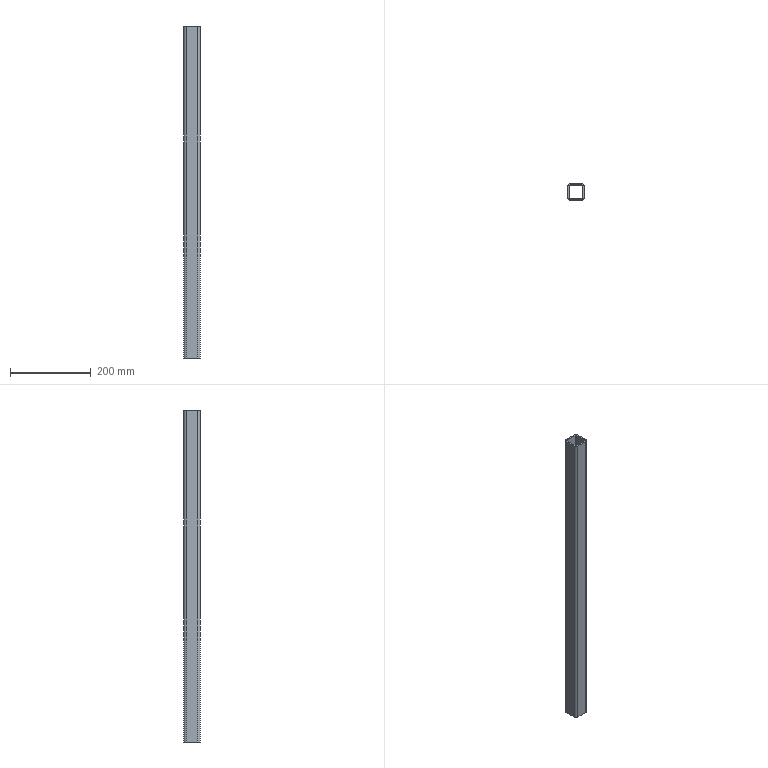Part | SolidWorks | features SavedExtBody 1 | 1 solid | 18 faces | box 40 x 40 x 820 mm | volume 364629 mm3 | plane 10 | cylinder 8 | commonest cylinder face diameters 6.4 x4 12.8 x4
STEP:
#1=CARTESIAN_POINT('',(-16.8,-13.6,410.));
#2=VERTEX_POINT('',#1);
#3=CARTESIAN_POINT('',(-16.8,-13.6,-410.));
#4=VERTEX_POINT('',#3);
#5=CARTESIAN_POINT('',(-16.8,-13.6,430.));
#6=DIRECTION('',(0.,0.,-1.));
#7=VECTOR('',#6,1000.);
#8=LINE('',#5,#7);
#9=EDGE_CURVE('',#2,#4,#8,.T.);
#10=ORIENTED_EDGE('',*,*,#9,.T.);
#11=CARTESIAN_POINT('',(-16.8,13.6,-410.));
#12=VERTEX_POINT('',#11);
#13=CARTESIAN_POINT('',(-16.8,-13.6,-410.));
#14=DIRECTION('',(0.,1.,0.));
#15=VECTOR('',#14,1000.);
#16=LINE('',#13,#15);
#17=EDGE_CURVE('',#4,#12,#16,.T.);
#18=ORIENTED_EDGE('',*,*,#17,.T.);
#19=CARTESIAN_POINT('',(-16.8,13.6,410.));
#20=VERTEX_POINT('',#19);
#21=CARTESIAN_POINT('',(-16.8,13.6,430.));
#22=DIRECTION('',(0.,0.,-1.));
#23=VECTOR('',#22,1000.);
#24=LINE('',#21,#23);
#25=EDGE_CURVE('',#20,#12,#24,.T.);
#26=ORIENTED_EDGE('',*,*,#25,.F.);
#27=CARTESIAN_POINT('',(-16.8,-13.6,410.));
#28=DIRECTION('',(0.,-1.,0.));
#29=VECTOR('',#28,1000.);
#30=LINE('',#27,#29);
#31=EDGE_CURVE('',#20,#2,#30,.T.);
#32=ORIENTED_EDGE('',*,*,#31,.T.);
#33=EDGE_LOOP('',(#10,#18,#26,#32));
#34=FACE_OUTER_BOUND('',#33,.T.);
#35=CARTESIAN_POINT('',(-16.8,-13.6,430.));
#36=DIRECTION('',(1.,0.,0.));
#37=DIRECTION('',(0.,1.,0.));
#38=AXIS2_PLACEMENT_3D('',#35,#36,#37);
#39=PLANE('',#38);
#40=ADVANCED_FACE('',(#34),#39,.T.);
#41=CARTESIAN_POINT('',(-13.6,-16.8,410.));
#42=VERTEX_POINT('',#41);
#43=CARTESIAN_POINT('',(-13.6,-16.8,-410.));
#44=VERTEX_POINT('',#43);
#45=CARTESIAN_POINT('',(-13.6,-16.8,430.));
#46=DIRECTION('',(0.,0.,-1.));
#47=VECTOR('',#46,1000.);
#48=LINE('',#45,#47);
#49=EDGE_CURVE('',#42,#44,#48,.T.);
#50=ORIENTED_EDGE('',*,*,#49,.T.);
#51=CARTESIAN_POINT('',(-13.6,-13.6,-410.));
#52=DIRECTION('',(0.,0.,-1.));
#53=DIRECTION('',(0.,1.,0.));
#54=AXIS2_PLACEMENT_3D('',#51,#52,#53);
#55=CIRCLE('',#54,3.2);
#56=EDGE_CURVE('',#44,#4,#55,.T.);
#57=ORIENTED_EDGE('',*,*,#56,.T.);
#58=ORIENTED_EDGE('',*,*,#9,.F.);
#59=CARTESIAN_POINT('',(-13.6,-13.6,410.));
#60=DIRECTION('',(0.,0.,1.));
#61=DIRECTION('',(0.,-1.,0.));
#62=AXIS2_PLACEMENT_3D('',#59,#60,#61);
#63=CIRCLE('',#62,3.2);
#64=EDGE_CURVE('',#2,#42,#63,.T.);
#65=ORIENTED_EDGE('',*,*,#64,.T.);
#66=EDGE_LOOP('',(#50,#57,#58,#65));
#67=FACE_OUTER_BOUND('',#66,.T.);
#68=CARTESIAN_POINT('',(-13.6,-13.6,430.));
#69=DIRECTION('',(0.,0.,-1.));
#70=DIRECTION('',(-1.,0.,0.));
#71=AXIS2_PLACEMENT_3D('',#68,#69,#70);
#72=CYLINDRICAL_SURFACE('',#71,3.2);
#73=ADVANCED_FACE('',(#67),#72,.F.);
#74=CARTESIAN_POINT('',(13.6,-16.8,410.));
#75=VERTEX_POINT('',#74);
#76=CARTESIAN_POINT('',(13.6,-16.8,-410.));
#77=VERTEX_POINT('',#76);
#78=CARTESIAN_POINT('',(13.6,-16.8,430.));
#79=DIRECTION('',(0.,0.,-1.));
#80=VECTOR('',#79,1000.);
#81=LINE('',#78,#80);
#82=EDGE_CURVE('',#75,#77,#81,.T.);
#83=ORIENTED_EDGE('',*,*,#82,.T.);
#84=CARTESIAN_POINT('',(-13.6,-16.8,-410.));
#85=DIRECTION('',(-1.,0.,0.));
#86=VECTOR('',#85,1000.);
#87=LINE('',#84,#86);
#88=EDGE_CURVE('',#77,#44,#87,.T.);
#89=ORIENTED_EDGE('',*,*,#88,.T.);
#90=ORIENTED_EDGE('',*,*,#49,.F.);
#91=CARTESIAN_POINT('',(-13.6,-16.8,410.));
#92=DIRECTION('',(1.,0.,0.));
#93=VECTOR('',#92,1000.);
#94=LINE('',#91,#93);
#95=EDGE_CURVE('',#42,#75,#94,.T.);
#96=ORIENTED_EDGE('',*,*,#95,.T.);
#97=EDGE_LOOP('',(#83,#89,#90,#96));
#98=FACE_OUTER_BOUND('',#97,.T.);
#99=CARTESIAN_POINT('',(-13.6,-16.8,430.));
#100=DIRECTION('',(0.,1.,0.));
#101=DIRECTION('',(-1.,0.,0.));
#102=AXIS2_PLACEMENT_3D('',#99,#100,#101);
#103=PLANE('',#102);
#104=ADVANCED_FACE('',(#98),#103,.T.);
#105=CARTESIAN_POINT('',(16.8,-13.6,410.));
#106=VERTEX_POINT('',#105);
#107=CARTESIAN_POINT('',(16.8,-13.6,-410.));
#108=VERTEX_POINT('',#107);
#109=CARTESIAN_POINT('',(16.8,-13.6,430.));
#110=DIRECTION('',(0.,0.,-1.));
#111=VECTOR('',#110,1000.);
#112=LINE('',#109,#111);
#113=EDGE_CURVE('',#106,#108,#112,.T.);
#114=ORIENTED_EDGE('',*,*,#113,.T.);
#115=CARTESIAN_POINT('',(13.6,-13.6,-410.));
#116=DIRECTION('',(0.,0.,-1.));
#117=DIRECTION('',(0.,1.,0.));
#118=AXIS2_PLACEMENT_3D('',#115,#116,#117);
#119=CIRCLE('',#118,3.2);
#120=EDGE_CURVE('',#108,#77,#119,.T.);
#121=ORIENTED_EDGE('',*,*,#120,.T.);
#122=ORIENTED_EDGE('',*,*,#82,.F.);
#123=CARTESIAN_POINT('',(13.6,-13.6,410.));
#124=DIRECTION('',(0.,0.,1.));
#125=DIRECTION('',(0.,-1.,0.));
#126=AXIS2_PLACEMENT_3D('',#123,#124,#125);
#127=CIRCLE('',#126,3.2);
#128=EDGE_CURVE('',#75,#106,#127,.T.);
#129=ORIENTED_EDGE('',*,*,#128,.T.);
#130=EDGE_LOOP('',(#114,#121,#122,#129));
#131=FACE_OUTER_BOUND('',#130,.T.);
#132=CARTESIAN_POINT('',(13.6,-13.6,430.));
#133=DIRECTION('',(0.,0.,-1.));
#134=DIRECTION('',(-1.,0.,0.));
#135=AXIS2_PLACEMENT_3D('',#132,#133,#134);
#136=CYLINDRICAL_SURFACE('',#135,3.2);
#137=ADVANCED_FACE('',(#131),#136,.F.);
#138=CARTESIAN_POINT('',(16.8,13.6,410.));
#139=VERTEX_POINT('',#138);
#140=CARTESIAN_POINT('',(16.8,13.6,-410.));
#141=VERTEX_POINT('',#140);
#142=CARTESIAN_POINT('',(16.8,13.6,430.));
#143=DIRECTION('',(0.,0.,-1.));
#144=VECTOR('',#143,1000.);
#145=LINE('',#142,#144);
#146=EDGE_CURVE('',#139,#141,#145,.T.);
#147=ORIENTED_EDGE('',*,*,#146,.T.);
#148=CARTESIAN_POINT('',(16.8,13.6,-410.));
#149=DIRECTION('',(0.,-1.,0.));
#150=VECTOR('',#149,1000.);
#151=LINE('',#148,#150);
#152=EDGE_CURVE('',#141,#108,#151,.T.);
#153=ORIENTED_EDGE('',*,*,#152,.T.);
#154=ORIENTED_EDGE('',*,*,#113,.F.);
#155=CARTESIAN_POINT('',(16.8,13.6,410.));
#156=DIRECTION('',(0.,1.,0.));
#157=VECTOR('',#156,1000.);
#158=LINE('',#155,#157);
#159=EDGE_CURVE('',#106,#139,#158,.T.);
#160=ORIENTED_EDGE('',*,*,#159,.T.);
#161=EDGE_LOOP('',(#147,#153,#154,#160));
#162=FACE_OUTER_BOUND('',#161,.T.);
#163=CARTESIAN_POINT('',(16.8,13.6,430.));
#164=DIRECTION('',(-1.,0.,0.));
#165=DIRECTION('',(0.,-1.,0.));
#166=AXIS2_PLACEMENT_3D('',#163,#164,#165);
#167=PLANE('',#166);
#168=ADVANCED_FACE('',(#162),#167,.T.);
#169=CARTESIAN_POINT('',(13.6,16.8,410.));
#170=VERTEX_POINT('',#169);
#171=CARTESIAN_POINT('',(13.6,16.8,-410.));
#172=VERTEX_POINT('',#171);
#173=CARTESIAN_POINT('',(13.6,16.8,430.));
#174=DIRECTION('',(0.,0.,-1.));
#175=VECTOR('',#174,1000.);
#176=LINE('',#173,#175);
#177=EDGE_CURVE('',#170,#172,#176,.T.);
#178=ORIENTED_EDGE('',*,*,#177,.T.);
#179=CARTESIAN_POINT('',(13.6,13.6,-410.));
#180=DIRECTION('',(0.,0.,-1.));
#181=DIRECTION('',(0.,1.,0.));
#182=AXIS2_PLACEMENT_3D('',#179,#180,#181);
#183=CIRCLE('',#182,3.2);
#184=EDGE_CURVE('',#172,#141,#183,.T.);
#185=ORIENTED_EDGE('',*,*,#184,.T.);
#186=ORIENTED_EDGE('',*,*,#146,.F.);
#187=CARTESIAN_POINT('',(13.6,13.6,410.));
#188=DIRECTION('',(0.,0.,1.));
#189=DIRECTION('',(0.,-1.,0.));
#190=AXIS2_PLACEMENT_3D('',#187,#188,#189);
#191=CIRCLE('',#190,3.2);
#192=EDGE_CURVE('',#139,#170,#191,.T.);
#193=ORIENTED_EDGE('',*,*,#192,.T.);
#194=EDGE_LOOP('',(#178,#185,#186,#193));
#195=FACE_OUTER_BOUND('',#194,.T.);
#196=CARTESIAN_POINT('',(13.6,13.6,430.));
#197=DIRECTION('',(0.,0.,-1.));
#198=DIRECTION('',(-1.,0.,0.));
#199=AXIS2_PLACEMENT_3D('',#196,#197,#198);
#200=CYLINDRICAL_SURFACE('',#199,3.2);
#201=ADVANCED_FACE('',(#195),#200,.F.);
#202=CARTESIAN_POINT('',(-13.6,16.8,410.));
#203=VERTEX_POINT('',#202);
#204=CARTESIAN_POINT('',(-13.6,16.8,-410.));
#205=VERTEX_POINT('',#204);
#206=CARTESIAN_POINT('',(-13.6,16.8,430.));
#207=DIRECTION('',(0.,0.,-1.));
#208=VECTOR('',#207,1000.);
#209=LINE('',#206,#208);
#210=EDGE_CURVE('',#203,#205,#209,.T.);
#211=ORIENTED_EDGE('',*,*,#210,.T.);
#212=CARTESIAN_POINT('',(13.6,16.8,-410.));
#213=DIRECTION('',(1.,0.,0.));
#214=VECTOR('',#213,1000.);
#215=LINE('',#212,#214);
#216=EDGE_CURVE('',#205,#172,#215,.T.);
#217=ORIENTED_EDGE('',*,*,#216,.T.);
#218=ORIENTED_EDGE('',*,*,#177,.F.);
#219=CARTESIAN_POINT('',(13.6,16.8,410.));
#220=DIRECTION('',(-1.,0.,0.));
#221=VECTOR('',#220,1000.);
#222=LINE('',#219,#221);
#223=EDGE_CURVE('',#170,#203,#222,.T.);
#224=ORIENTED_EDGE('',*,*,#223,.T.);
#225=EDGE_LOOP('',(#211,#217,#218,#224));
#226=FACE_OUTER_BOUND('',#225,.T.);
#227=CARTESIAN_POINT('',(13.6,16.8,430.));
#228=DIRECTION('',(0.,-1.,0.));
#229=DIRECTION('',(1.,0.,0.));
#230=AXIS2_PLACEMENT_3D('',#227,#228,#229);
#231=PLANE('',#230);
#232=ADVANCED_FACE('',(#226),#231,.T.);
#233=ORIENTED_EDGE('',*,*,#25,.T.);
#234=CARTESIAN_POINT('',(-13.6,13.6,-410.));
#235=DIRECTION('',(0.,0.,-1.));
#236=DIRECTION('',(0.,1.,0.));
#237=AXIS2_PLACEMENT_3D('',#234,#235,#236);
#238=CIRCLE('',#237,3.2);
#239=EDGE_CURVE('',#12,#205,#238,.T.);
#240=ORIENTED_EDGE('',*,*,#239,.T.);
#241=ORIENTED_EDGE('',*,*,#210,.F.);
#242=CARTESIAN_POINT('',(-13.6,13.6,410.));
#243=DIRECTION('',(0.,0.,1.));
#244=DIRECTION('',(0.,-1.,0.));
#245=AXIS2_PLACEMENT_3D('',#242,#243,#244);
#246=CIRCLE('',#245,3.2);
#247=EDGE_CURVE('',#203,#20,#246,.T.);
#248=ORIENTED_EDGE('',*,*,#247,.T.);
#249=EDGE_LOOP('',(#233,#240,#241,#248));
#250=FACE_OUTER_BOUND('',#249,.T.);
#251=CARTESIAN_POINT('',(-13.6,13.6,430.));
#252=DIRECTION('',(0.,0.,-1.));
#253=DIRECTION('',(-1.,0.,0.));
#254=AXIS2_PLACEMENT_3D('',#251,#252,#253);
#255=CYLINDRICAL_SURFACE('',#254,3.2);
#256=ADVANCED_FACE('',(#250),#255,.F.);
#257=ORIENTED_EDGE('',*,*,#223,.F.);
#258=ORIENTED_EDGE('',*,*,#192,.F.);
#259=ORIENTED_EDGE('',*,*,#159,.F.);
#260=ORIENTED_EDGE('',*,*,#128,.F.);
#261=ORIENTED_EDGE('',*,*,#95,.F.);
#262=ORIENTED_EDGE('',*,*,#64,.F.);
#263=ORIENTED_EDGE('',*,*,#31,.F.);
#264=ORIENTED_EDGE('',*,*,#247,.F.);
#265=EDGE_LOOP('',(#257,#258,#259,#260,#261,#262,#263,#264));
#266=FACE_BOUND('',#265,.T.);
#267=CARTESIAN_POINT('',(20.,13.6,410.));
#268=VERTEX_POINT('',#267);
#269=CARTESIAN_POINT('',(13.6,20.,410.));
#270=VERTEX_POINT('',#269);
#271=CARTESIAN_POINT('',(13.6,13.6,410.));
#272=DIRECTION('',(0.,0.,1.));
#273=DIRECTION('',(0.,-1.,0.));
#274=AXIS2_PLACEMENT_3D('',#271,#272,#273);
#275=CIRCLE('',#274,6.4);
#276=EDGE_CURVE('',#268,#270,#275,.T.);
#277=ORIENTED_EDGE('',*,*,#276,.T.);
#278=CARTESIAN_POINT('',(-13.6,20.,410.));
#279=VERTEX_POINT('',#278);
#280=CARTESIAN_POINT('',(13.6,20.,410.));
#281=DIRECTION('',(-1.,0.,0.));
#282=VECTOR('',#281,1000.);
#283=LINE('',#280,#282);
#284=EDGE_CURVE('',#270,#279,#283,.T.);
#285=ORIENTED_EDGE('',*,*,#284,.T.);
#286=CARTESIAN_POINT('',(-20.,13.6,410.));
#287=VERTEX_POINT('',#286);
#288=CARTESIAN_POINT('',(-13.6,13.6,410.));
#289=DIRECTION('',(0.,0.,1.));
#290=DIRECTION('',(0.,-1.,0.));
#291=AXIS2_PLACEMENT_3D('',#288,#289,#290);
#292=CIRCLE('',#291,6.4);
#293=EDGE_CURVE('',#279,#287,#292,.T.);
#294=ORIENTED_EDGE('',*,*,#293,.T.);
#295=CARTESIAN_POINT('',(-20.,-13.6,410.));
#296=VERTEX_POINT('',#295);
#297=CARTESIAN_POINT('',(-20.,-320.,410.));
#298=DIRECTION('',(0.,1.,0.));
#299=VECTOR('',#298,1000.);
#300=LINE('',#297,#299);
#301=EDGE_CURVE('',#296,#287,#300,.T.);
#302=ORIENTED_EDGE('',*,*,#301,.F.);
#303=CARTESIAN_POINT('',(-13.6,-20.,410.));
#304=VERTEX_POINT('',#303);
#305=CARTESIAN_POINT('',(-13.6,-13.6,410.));
#306=DIRECTION('',(0.,0.,1.));
#307=DIRECTION('',(0.,-1.,0.));
#308=AXIS2_PLACEMENT_3D('',#305,#306,#307);
#309=CIRCLE('',#308,6.4);
#310=EDGE_CURVE('',#296,#304,#309,.T.);
#311=ORIENTED_EDGE('',*,*,#310,.T.);
#312=CARTESIAN_POINT('',(13.6,-20.,410.));
#313=VERTEX_POINT('',#312);
#314=CARTESIAN_POINT('',(-13.6,-20.,410.));
#315=DIRECTION('',(1.,0.,0.));
#316=VECTOR('',#315,1000.);
#317=LINE('',#314,#316);
#318=EDGE_CURVE('',#304,#313,#317,.T.);
#319=ORIENTED_EDGE('',*,*,#318,.T.);
#320=CARTESIAN_POINT('',(20.,-13.6,410.));
#321=VERTEX_POINT('',#320);
#322=CARTESIAN_POINT('',(13.6,-13.6,410.));
#323=DIRECTION('',(0.,0.,1.));
#324=DIRECTION('',(0.,-1.,0.));
#325=AXIS2_PLACEMENT_3D('',#322,#323,#324);
#326=CIRCLE('',#325,6.4);
#327=EDGE_CURVE('',#313,#321,#326,.T.);
#328=ORIENTED_EDGE('',*,*,#327,.T.);
#329=CARTESIAN_POINT('',(20.,13.6,410.));
#330=DIRECTION('',(0.,1.,0.));
#331=VECTOR('',#330,1000.);
#332=LINE('',#329,#331);
#333=EDGE_CURVE('',#321,#268,#332,.T.);
#334=ORIENTED_EDGE('',*,*,#333,.T.);
#335=EDGE_LOOP('',(#277,#285,#294,#302,#311,#319,#328,#334));
#336=FACE_OUTER_BOUND('',#335,.T.);
#337=CARTESIAN_POINT('',(-13.6,-320.,410.));
#338=DIRECTION('',(0.,0.,1.));
#339=DIRECTION('',(0.,-1.,0.));
#340=AXIS2_PLACEMENT_3D('',#337,#338,#339);
#341=PLANE('',#340);
#342=ADVANCED_FACE('',(#266,#336),#341,.T.);
#343=CARTESIAN_POINT('',(20.,13.6,-410.));
#344=VERTEX_POINT('',#343);
#345=CARTESIAN_POINT('',(20.,-13.6,-410.));
#346=VERTEX_POINT('',#345);
#347=CARTESIAN_POINT('',(20.,13.6,-410.));
#348=DIRECTION('',(0.,-1.,0.));
#349=VECTOR('',#348,1000.);
#350=LINE('',#347,#349);
#351=EDGE_CURVE('',#344,#346,#350,.T.);
#352=ORIENTED_EDGE('',*,*,#351,.F.);
#353=CARTESIAN_POINT('',(20.,13.6,430.));
#354=DIRECTION('',(0.,0.,-1.));
#355=VECTOR('',#354,1000.);
#356=LINE('',#353,#355);
#357=EDGE_CURVE('',#268,#344,#356,.T.);
#358=ORIENTED_EDGE('',*,*,#357,.F.);
#359=ORIENTED_EDGE('',*,*,#333,.F.);
#360=CARTESIAN_POINT('',(20.,-13.6,430.));
#361=DIRECTION('',(0.,0.,-1.));
#362=VECTOR('',#361,1000.);
#363=LINE('',#360,#362);
#364=EDGE_CURVE('',#321,#346,#363,.T.);
#365=ORIENTED_EDGE('',*,*,#364,.T.);
#366=EDGE_LOOP('',(#352,#358,#359,#365));
#367=FACE_OUTER_BOUND('',#366,.T.);
#368=CARTESIAN_POINT('',(20.,13.6,430.));
#369=DIRECTION('',(-1.,0.,0.));
#370=DIRECTION('',(0.,-1.,0.));
#371=AXIS2_PLACEMENT_3D('',#368,#369,#370);
#372=PLANE('',#371);
#373=ADVANCED_FACE('',(#367),#372,.F.);
#374=CARTESIAN_POINT('',(13.6,-20.,-410.));
#375=VERTEX_POINT('',#374);
#376=CARTESIAN_POINT('',(13.6,-13.6,-410.));
#377=DIRECTION('',(0.,0.,-1.));
#378=DIRECTION('',(0.,1.,0.));
#379=AXIS2_PLACEMENT_3D('',#376,#377,#378);
#380=CIRCLE('',#379,6.4);
#381=EDGE_CURVE('',#346,#375,#380,.T.);
#382=ORIENTED_EDGE('',*,*,#381,.F.);
#383=ORIENTED_EDGE('',*,*,#364,.F.);
#384=ORIENTED_EDGE('',*,*,#327,.F.);
#385=CARTESIAN_POINT('',(13.6,-20.,430.));
#386=DIRECTION('',(0.,0.,-1.));
#387=VECTOR('',#386,1000.);
#388=LINE('',#385,#387);
#389=EDGE_CURVE('',#313,#375,#388,.T.);
#390=ORIENTED_EDGE('',*,*,#389,.T.);
#391=EDGE_LOOP('',(#382,#383,#384,#390));
#392=FACE_OUTER_BOUND('',#391,.T.);
#393=CARTESIAN_POINT('',(13.6,-13.6,430.));
#394=DIRECTION('',(0.,0.,-1.));
#395=DIRECTION('',(-1.,0.,0.));
#396=AXIS2_PLACEMENT_3D('',#393,#394,#395);
#397=CYLINDRICAL_SURFACE('',#396,6.4);
#398=ADVANCED_FACE('',(#392),#397,.T.);
#399=CARTESIAN_POINT('',(-13.6,-20.,-410.));
#400=VERTEX_POINT('',#399);
#401=CARTESIAN_POINT('',(-13.6,-20.,-410.));
#402=DIRECTION('',(-1.,0.,0.));
#403=VECTOR('',#402,1000.);
#404=LINE('',#401,#403);
#405=EDGE_CURVE('',#375,#400,#404,.T.);
#406=ORIENTED_EDGE('',*,*,#405,.F.);
#407=ORIENTED_EDGE('',*,*,#389,.F.);
#408=ORIENTED_EDGE('',*,*,#318,.F.);
#409=CARTESIAN_POINT('',(-13.6,-20.,430.));
#410=DIRECTION('',(0.,0.,-1.));
#411=VECTOR('',#410,1000.);
#412=LINE('',#409,#411);
#413=EDGE_CURVE('',#304,#400,#412,.T.);
#414=ORIENTED_EDGE('',*,*,#413,.T.);
#415=EDGE_LOOP('',(#406,#407,#408,#414));
#416=FACE_OUTER_BOUND('',#415,.T.);
#417=CARTESIAN_POINT('',(-13.6,-20.,430.));
#418=DIRECTION('',(0.,1.,0.));
#419=DIRECTION('',(-1.,0.,0.));
#420=AXIS2_PLACEMENT_3D('',#417,#418,#419);
#421=PLANE('',#420);
#422=ADVANCED_FACE('',(#416),#421,.F.);
#423=CARTESIAN_POINT('',(-20.,-13.6,-410.));
#424=VERTEX_POINT('',#423);
#425=CARTESIAN_POINT('',(-13.6,-13.6,-410.));
#426=DIRECTION('',(0.,0.,-1.));
#427=DIRECTION('',(0.,1.,0.));
#428=AXIS2_PLACEMENT_3D('',#425,#426,#427);
#429=CIRCLE('',#428,6.4);
#430=EDGE_CURVE('',#400,#424,#429,.T.);
#431=ORIENTED_EDGE('',*,*,#430,.F.);
#432=ORIENTED_EDGE('',*,*,#413,.F.);
#433=ORIENTED_EDGE('',*,*,#310,.F.);
#434=CARTESIAN_POINT('',(-20.,-13.6,430.));
#435=DIRECTION('',(0.,0.,-1.));
#436=VECTOR('',#435,1000.);
#437=LINE('',#434,#436);
#438=EDGE_CURVE('',#296,#424,#437,.T.);
#439=ORIENTED_EDGE('',*,*,#438,.T.);
#440=EDGE_LOOP('',(#431,#432,#433,#439));
#441=FACE_OUTER_BOUND('',#440,.T.);
#442=CARTESIAN_POINT('',(-13.6,-13.6,430.));
#443=DIRECTION('',(0.,0.,-1.));
#444=DIRECTION('',(-1.,0.,0.));
#445=AXIS2_PLACEMENT_3D('',#442,#443,#444);
#446=CYLINDRICAL_SURFACE('',#445,6.4);
#447=ADVANCED_FACE('',(#441),#446,.T.);
#448=CARTESIAN_POINT('',(-20.,13.6,-410.));
#449=VERTEX_POINT('',#448);
#450=CARTESIAN_POINT('',(-20.,-320.,-410.));
#451=DIRECTION('',(0.,1.,0.));
#452=VECTOR('',#451,1000.);
#453=LINE('',#450,#452);
#454=EDGE_CURVE('',#424,#449,#453,.T.);
#455=ORIENTED_EDGE('',*,*,#454,.F.);
#456=ORIENTED_EDGE('',*,*,#438,.F.);
#457=ORIENTED_EDGE('',*,*,#301,.T.);
#458=CARTESIAN_POINT('',(-20.,13.6,430.));
#459=DIRECTION('',(0.,0.,-1.));
#460=VECTOR('',#459,1000.);
#461=LINE('',#458,#460);
#462=EDGE_CURVE('',#287,#449,#461,.T.);
#463=ORIENTED_EDGE('',*,*,#462,.T.);
#464=EDGE_LOOP('',(#455,#456,#457,#463));
#465=FACE_OUTER_BOUND('',#464,.T.);
#466=CARTESIAN_POINT('',(-20.,-13.6,430.));
#467=DIRECTION('',(1.,0.,0.));
#468=DIRECTION('',(0.,1.,0.));
#469=AXIS2_PLACEMENT_3D('',#466,#467,#468);
#470=PLANE('',#469);
#471=ADVANCED_FACE('',(#465),#470,.F.);
#472=CARTESIAN_POINT('',(-13.6,20.,-410.));
#473=VERTEX_POINT('',#472);
#474=CARTESIAN_POINT('',(-13.6,13.6,-410.));
#475=DIRECTION('',(0.,0.,-1.));
#476=DIRECTION('',(0.,1.,0.));
#477=AXIS2_PLACEMENT_3D('',#474,#475,#476);
#478=CIRCLE('',#477,6.4);
#479=EDGE_CURVE('',#449,#473,#478,.T.);
#480=ORIENTED_EDGE('',*,*,#479,.F.);
#481=ORIENTED_EDGE('',*,*,#462,.F.);
#482=ORIENTED_EDGE('',*,*,#293,.F.);
#483=CARTESIAN_POINT('',(-13.6,20.,430.));
#484=DIRECTION('',(0.,0.,-1.));
#485=VECTOR('',#484,1000.);
#486=LINE('',#483,#485);
#487=EDGE_CURVE('',#279,#473,#486,.T.);
#488=ORIENTED_EDGE('',*,*,#487,.T.);
#489=EDGE_LOOP('',(#480,#481,#482,#488));
#490=FACE_OUTER_BOUND('',#489,.T.);
#491=CARTESIAN_POINT('',(-13.6,13.6,430.));
#492=DIRECTION('',(0.,0.,-1.));
#493=DIRECTION('',(-1.,0.,0.));
#494=AXIS2_PLACEMENT_3D('',#491,#492,#493);
#495=CYLINDRICAL_SURFACE('',#494,6.4);
#496=ADVANCED_FACE('',(#490),#495,.T.);
#497=CARTESIAN_POINT('',(13.6,20.,-410.));
#498=VERTEX_POINT('',#497);
#499=CARTESIAN_POINT('',(13.6,20.,-410.));
#500=DIRECTION('',(1.,0.,0.));
#501=VECTOR('',#500,1000.);
#502=LINE('',#499,#501);
#503=EDGE_CURVE('',#473,#498,#502,.T.);
#504=ORIENTED_EDGE('',*,*,#503,.F.);
#505=ORIENTED_EDGE('',*,*,#487,.F.);
#506=ORIENTED_EDGE('',*,*,#284,.F.);
#507=CARTESIAN_POINT('',(13.6,20.,430.));
#508=DIRECTION('',(0.,0.,-1.));
#509=VECTOR('',#508,1000.);
#510=LINE('',#507,#509);
#511=EDGE_CURVE('',#270,#498,#510,.T.);
#512=ORIENTED_EDGE('',*,*,#511,.T.);
#513=EDGE_LOOP('',(#504,#505,#506,#512));
#514=FACE_OUTER_BOUND('',#513,.T.);
#515=CARTESIAN_POINT('',(13.6,20.,430.));
#516=DIRECTION('',(0.,-1.,0.));
#517=DIRECTION('',(1.,0.,0.));
#518=AXIS2_PLACEMENT_3D('',#515,#516,#517);
#519=PLANE('',#518);
#520=ADVANCED_FACE('',(#514),#519,.F.);
#521=CARTESIAN_POINT('',(13.6,13.6,-410.));
#522=DIRECTION('',(0.,0.,-1.));
#523=DIRECTION('',(0.,1.,0.));
#524=AXIS2_PLACEMENT_3D('',#521,#522,#523);
#525=CIRCLE('',#524,6.4);
#526=EDGE_CURVE('',#498,#344,#525,.T.);
#527=ORIENTED_EDGE('',*,*,#526,.F.);
#528=ORIENTED_EDGE('',*,*,#511,.F.);
#529=ORIENTED_EDGE('',*,*,#276,.F.);
#530=ORIENTED_EDGE('',*,*,#357,.T.);
#531=EDGE_LOOP('',(#527,#528,#529,#530));
#532=FACE_OUTER_BOUND('',#531,.T.);
#533=CARTESIAN_POINT('',(13.6,13.6,430.));
#534=DIRECTION('',(0.,0.,-1.));
#535=DIRECTION('',(-1.,0.,0.));
#536=AXIS2_PLACEMENT_3D('',#533,#534,#535);
#537=CYLINDRICAL_SURFACE('',#536,6.4);
#538=ADVANCED_FACE('',(#532),#537,.T.);
#539=ORIENTED_EDGE('',*,*,#17,.F.);
#540=ORIENTED_EDGE('',*,*,#56,.F.);
#541=ORIENTED_EDGE('',*,*,#88,.F.);
#542=ORIENTED_EDGE('',*,*,#120,.F.);
#543=ORIENTED_EDGE('',*,*,#152,.F.);
#544=ORIENTED_EDGE('',*,*,#184,.F.);
#545=ORIENTED_EDGE('',*,*,#216,.F.);
#546=ORIENTED_EDGE('',*,*,#239,.F.);
#547=EDGE_LOOP('',(#539,#540,#541,#542,#543,#544,#545,#546));
#548=FACE_BOUND('',#547,.T.);
#549=ORIENTED_EDGE('',*,*,#526,.T.);
#550=ORIENTED_EDGE('',*,*,#351,.T.);
#551=ORIENTED_EDGE('',*,*,#381,.T.);
#552=ORIENTED_EDGE('',*,*,#405,.T.);
#553=ORIENTED_EDGE('',*,*,#430,.T.);
#554=ORIENTED_EDGE('',*,*,#454,.T.);
#555=ORIENTED_EDGE('',*,*,#479,.T.);
#556=ORIENTED_EDGE('',*,*,#503,.T.);
#557=EDGE_LOOP('',(#549,#550,#551,#552,#553,#554,#555,#556));
#558=FACE_OUTER_BOUND('',#557,.T.);
#559=CARTESIAN_POINT('',(13.6,-320.,-410.));
#560=DIRECTION('',(0.,0.,-1.));
#561=DIRECTION('',(0.,1.,0.));
#562=AXIS2_PLACEMENT_3D('',#559,#560,#561);
#563=PLANE('',#562);
#564=ADVANCED_FACE('',(#548,#558),#563,.T.);
#565=CLOSED_SHELL('',(#40,#73,#104,#137,#168,#201,#232,#256,#342,#373,#398,#422,#447,#471,#496,#520,#538,#564));
#566=MANIFOLD_SOLID_BREP('',#565);
#567=CARTESIAN_POINT('',(0.,0.,0.));
#568=DIRECTION('',(0.,0.,1.));
#569=DIRECTION('',(1.,0.,0.));
#570=AXIS2_PLACEMENT_3D('',#567,#568,#569);
#571=(LENGTH_UNIT()NAMED_UNIT(*)SI_UNIT(.MILLI.,.METRE.));
#572=UNCERTAINTY_MEASURE_WITH_UNIT(LENGTH_MEASURE(0.00001),#571,'','');
#573=(NAMED_UNIT(*)PLANE_ANGLE_UNIT()SI_UNIT($,.RADIAN.));
#574=(NAMED_UNIT(*)SI_UNIT($,.STERADIAN.)SOLID_ANGLE_UNIT());
#575=(GEOMETRIC_REPRESENTATION_CONTEXT(3)GLOBAL_UNCERTAINTY_ASSIGNED_CONTEXT((#572))GLOBAL_UNIT_ASSIGNED_CONTEXT((#571,#573,#574))REPRESENTATION_CONTEXT('',''));
#576=ADVANCED_BREP_SHAPE_REPRESENTATION('',(#566,#570),#575);